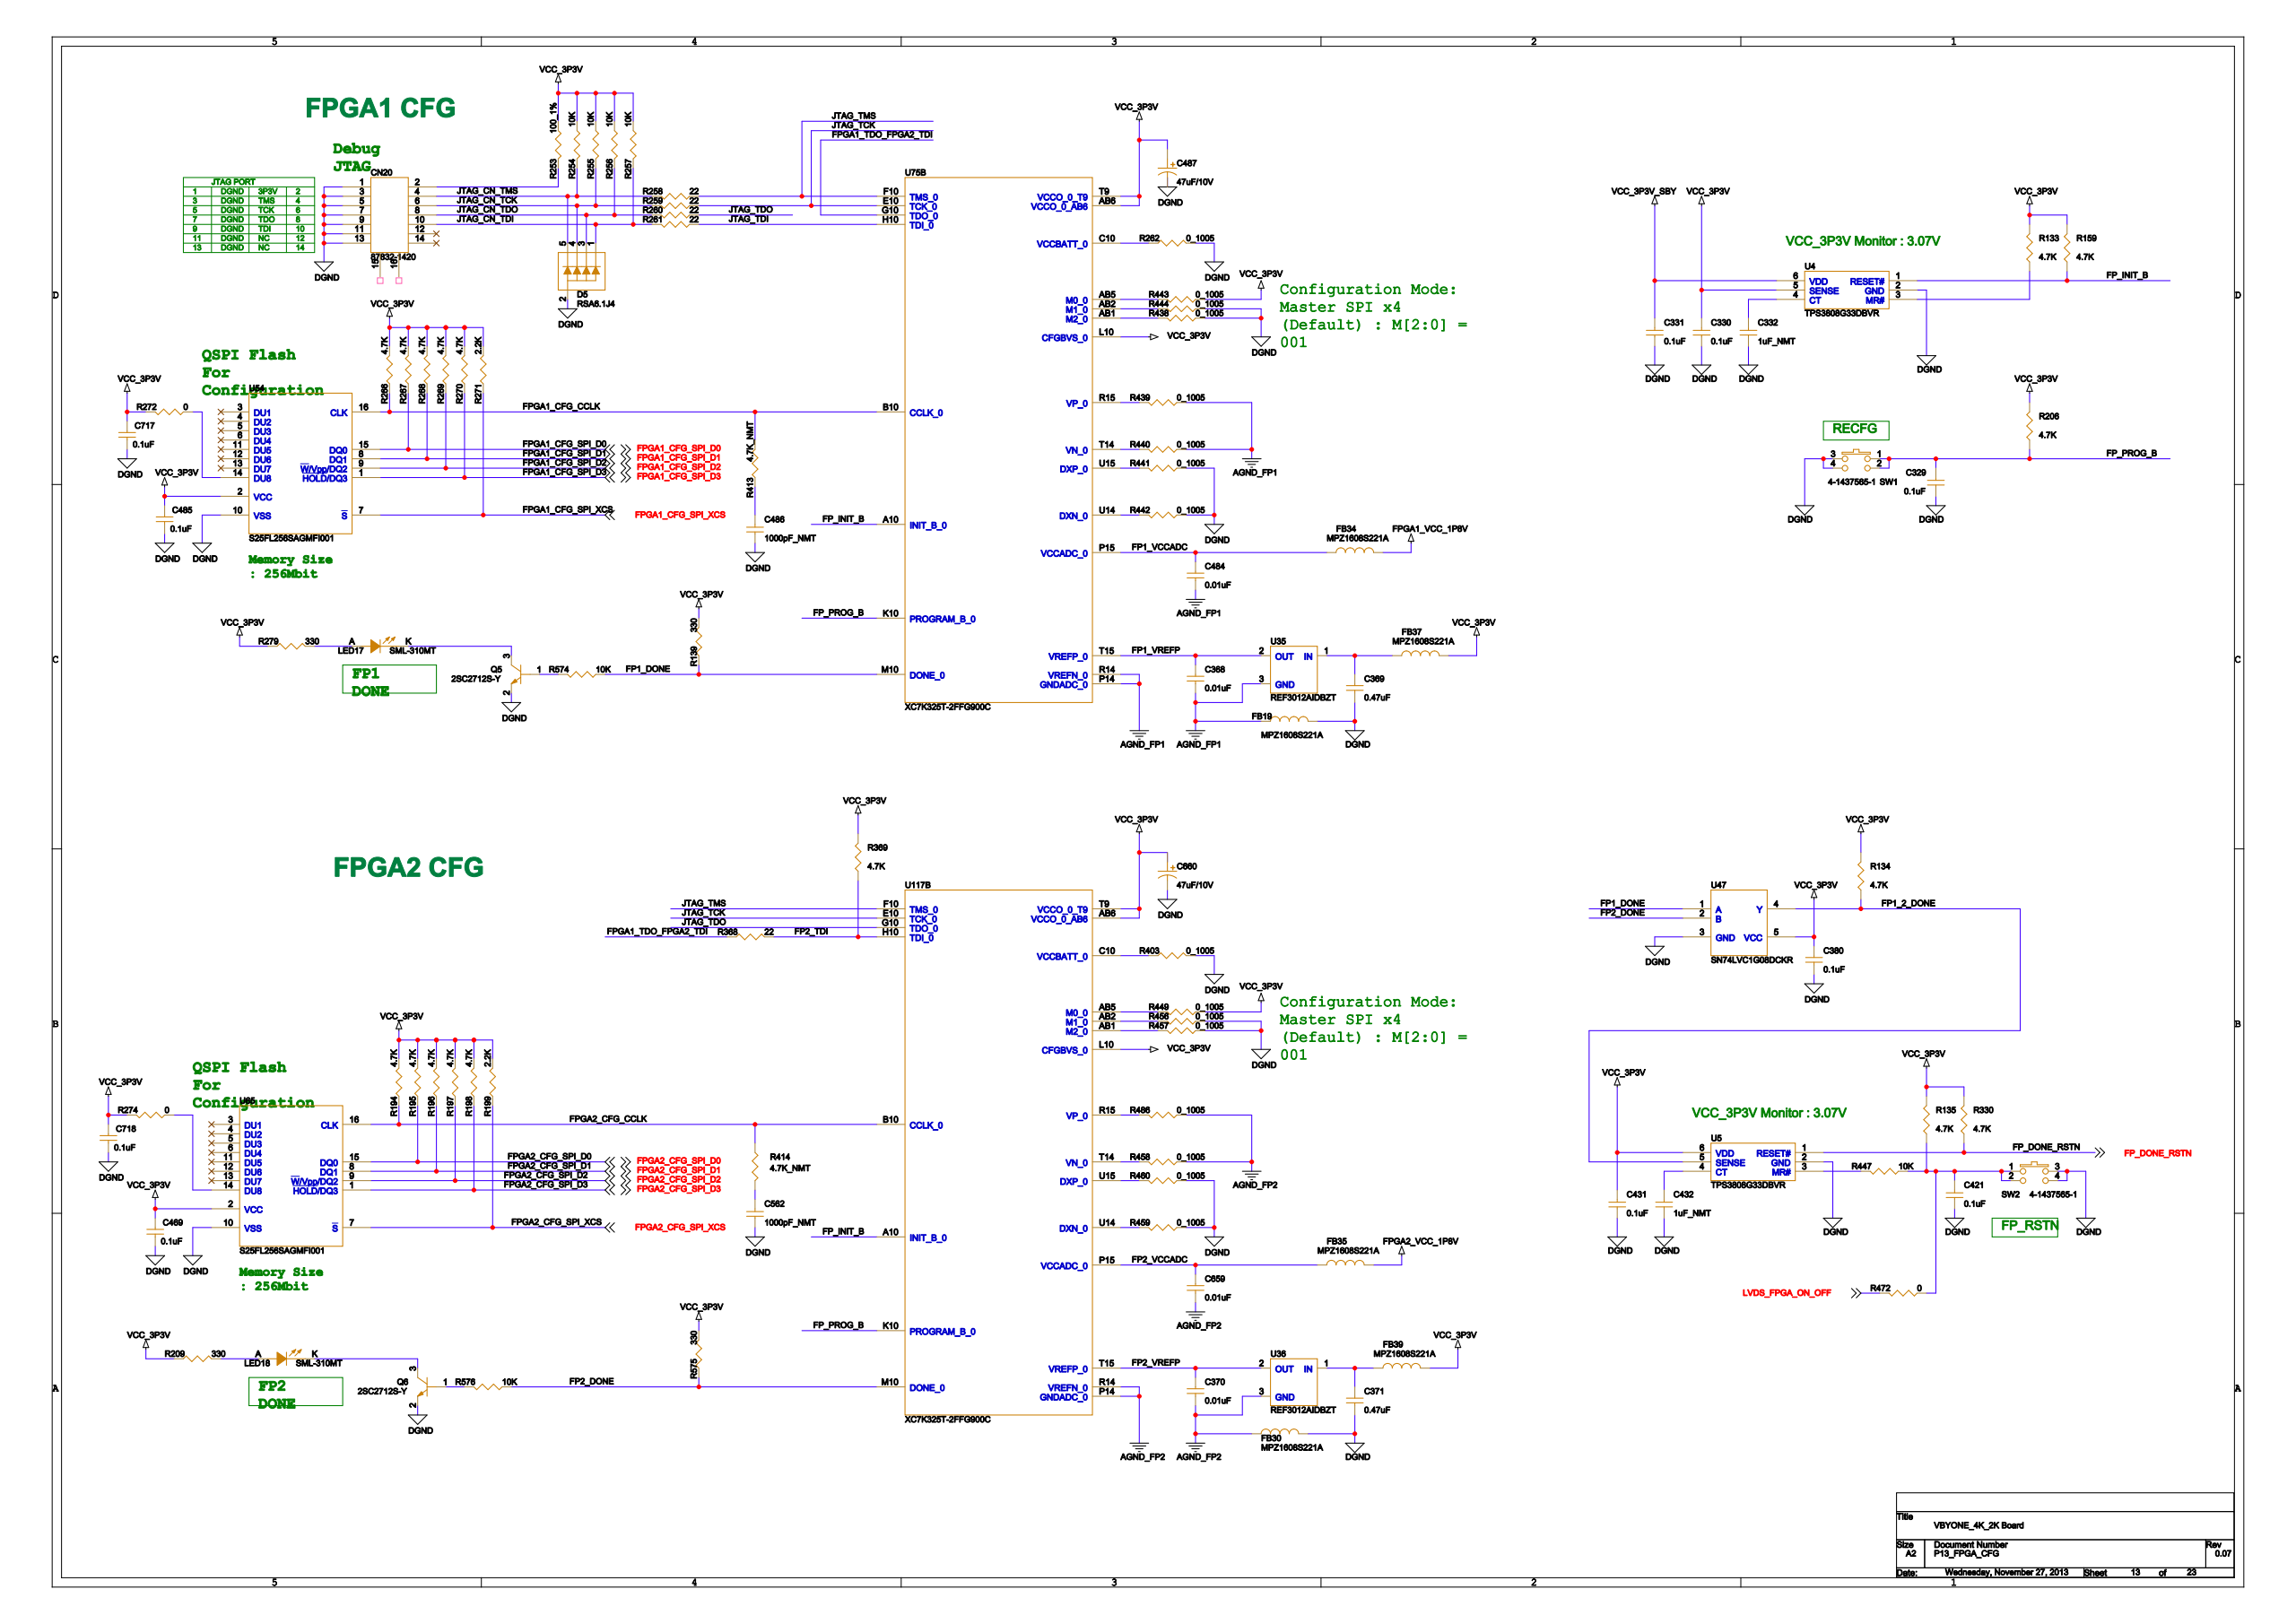Circuit board | Cadence Allegro | 1712 parts | 1495 nets | one sheet of the schematic
Parts on this sheet (reference | value | footprint):
C329 | 0.1uF | CRC1005RZAS
C330 | 0.1uF | CRC1005RZAS
C331 | 0.1uF | CRC1005RZAS
C332 | 1uF_NMT | CRC1608RZAS
C368 | 0.01uF | CRC1005RZAS
C369 | 0.47uF | CRC1608RZAS
C370 | 0.01uF | CRC1005RZAS
C371 | 0.47uF | CRC1608RZAS
C380 | 0.1uF | CRC1005RZAS
C421 | 0.1uF | CRC1005RZAS
C431 | 0.1uF | CRC1005RZAS
C432 | 1uF_NMT | CRC1608RZAS
C469 | 0.1uF | CRC1005RZAS
C484 | 0.01uF | CRC1005RZAS
C485 | 0.1uF | CRC1005RZAS
C486 | 1000pF_NMT | CRC1608RZAS
C487 | 47uF/10V | CEC3528RZAS
C562 | 1000pF_NMT | CRC1608RZAS
C659 | 0.01uF | CRC1005RZAS
C660 | 47uF/10V | CEC3528RZAS
C717 | 0.1uF | CRC1005RZAS
C718 | 0.1uF | CRC1005RZAS
CN20 | 87832-1420 | CNC014RJAS
D5 | RSA6.1J4 | DIC005RCAS
FB19 | MPZ1608S221A | LSC1608RZAS
FB30 | MPZ1608S221A | LSC1608RZAS
FB34 | MPZ1608S221A | LSC1608RZAS
FB35 | MPZ1608S221A | LSC1608RZAS
FB37 | MPZ1608S221A | LSC1608RZAS
FB39 | MPZ1608S221A | LSC1608RZAS
LED17 | SML-310MT | LEC1608RZAS
LED18 | SML-310MT | LEC1608RZAS
Q5 | 2SC2712S-Y | TRC003RZCS
Q6 | 2SC2712S-Y | TRC003RZCS
R133 | 4.7K | CRC1005RZAS
R134 | 4.7K | CRC1005RZAS
R135 | 4.7K | CRC1005RZAS
R139 | 330 | CRC1608RZAS
R159 | 4.7K | CRC1005RZAS
R194 | 4.7K | CRC1005RZAS
R195 | 4.7K | CRC1005RZAS
R196 | 4.7K | CRC1005RZAS
R197 | 4.7K | CRC1005RZAS
R198 | 4.7K | CRC1005RZAS
R199 | 2.2K | CRC1005RZAS
R206 | 4.7K | CRC1005RZAS
R209 | 330 | CRC1608RZAS
R253 | 100_1% | CRC1005RZAS
R254 | 10K | CRC1005RZAS
R255 | 10K | CRC1005RZAS
R256 | 10K | CRC1005RZAS
R257 | 10K | CRC1005RZAS
R258 | 22 | CRC1005RZAS
R259 | 22 | CRC1005RZAS
R260 | 22 | CRC1005RZAS
R261 | 22 | CRC1005RZAS
R262 | 0_1005 | CRC1005RZAS
R266 | 4.7K | CRC1005RZAS
R267 | 4.7K | CRC1005RZAS
R268 | 4.7K | CRC1005RZAS
R269 | 4.7K | CRC1005RZAS
R270 | 4.7K | CRC1005RZAS
R271 | 2.2K | CRC1005RZAS
R272 | 0 | CRC1608RZAS
R274 | 0 | CRC1608RZAS
R279 | 330 | CRC1608RZAS
R330 | 4.7K | CRC1005RZAS
R368 | 22 | CRC1005RZAS
R369 | 4.7K | CRC1005RZAS
R403 | 0_1005 | CRC1005RZAS
R413 | 4.7K_NMT | CRC1608RZAS
R414 | 4.7K_NMT | CRC1608RZAS
R438 | 0_1005 | CRC1005RZAS
R439 | 0_1005 | CRC1005RZAS
R440 | 0_1005 | CRC1005RZAS
R441 | 0_1005 | CRC1005RZAS
R442 | 0_1005 | CRC1005RZAS
R443 | 0_1005 | CRC1005RZAS
R444 | 0_1005 | CRC1005RZAS
R447 | 10K | CRC1005RZAS
R449 | 0_1005 | CRC1005RZAS
R456 | 0_1005 | CRC1005RZAS
R457 | 0_1005 | CRC1005RZAS
R458 | 0_1005 | CRC1005RZAS
R459 | 0_1005 | CRC1005RZAS
R460 | 0_1005 | CRC1005RZAS
R472 | 0 | CRC1608RZAS
R486 | 0_1005 | CRC1005RZAS
R574 | 10K | CRC1005RZAS
R575 | 330 | CRC1608RZAS
R576 | 10K | CRC1005RZAS
SW1 | 4-1437565-1 | SWC004RZBS
SW2 | 4-1437565-1 | SWC004RZBS
U4 | TPS3808G33DBVR | SOC006RZBS
U5 | TPS3808G33DBVR | SOC006RZBS
U15 | SII1161CTU | QFP100RCBS
U35 | REF3012AIDBZT | TRC003RZGS
U36 | REF3012AIDBZT | TRC003RZGS
U47 | SN74LVC1G08DCKR | SOC005REAS
U54 | S25FL256SAGMFI001 | SOC016RHAS
U65 | S25FL256SAGMFI001 | SOC016RHAS
U75 | XC7K325T-2FFG900C | BGA900RGAS
U117 | XC7K325T-2FFG900C | BGA900RGAS
Nets of these parts (net: part-pin ...):
VCC_3P3V: C330-2 C380-1 C431-2 C469-1 C485-1 C487-1 C660-1 C717-1 C718-1 FB37-2 FB39-2 R133-2 R134-2 R135-2 R139-2 R159-2 R194-1 R195-1 R196-1 R197-1 R198-1 R199-1 R206-2 R209-2 R253-2 R254-1 R255-1 R256-1 R257-1 R266-1 R267-1 R268-1 R269-1 R270-1 R271-1 R272-1 R274-1 R279-2 R330-2 R369-2 R443-1 R449-1 R575-2 U4-5 U5-6 U47-5 U54-2 U65-2 U15-2 U15-9 U75-AB6 U75-L10 U75-T9 U117-AB6 U117-L10 U117-T9
DGND: C329-1 C330-1 C331-1 C332-1 C369-2 C371-2 C380-2 C421-1 C431-1 C432-1 C469-2 C485-2 C486-1 C487-2 C562-1 C660-2 C717-2 C718-2 CN20-1 CN20-3 CN20-5 CN20-7 CN20-9 CN20-11 CN20-13 D5-2 FB19-2 FB30-2 Q5-2 Q6-2 R262-2 R403-2 R438-1 R441-1 R442-1 R444-1 R456-1 R457-1 R459-1 R460-1 SW1-3 SW1-4 SW2-3 SW2-4 U4-2 U5-2 U47-3 U54-10 U65-10 U15-5 U75-A2 U75-D5 U117-A2
VCC_3P3V_SBY: C331-2 U4-6
FPGA1_VCC_1P8V: FB34-2
FPGA2_VCC_1P8V: FB35-2
FP_PROG_B: C329-2 R206-1 SW1-1 SW1-2 U75-K10 U117-K10
N17557052: C421-2 R135-1 R447-1 R472-1 SW2-1 SW2-2
N17490659: C332-2 U4-4
N17557080: C432-2 U5-4
FP1_VREFP: C368-1 U35-2 U75-T15
AGND_FP1: C368-2 C484-2 FB19-1 R439-1 R440-1 U35-3 U75-P14 U75-R14
FP2_VREFP: C370-1 U36-2 U117-T15
AGND_FP2: C370-2 C659-2 FB30-1 R458-1 R486-1 U36-3 U117-P14 U117-R14
N18104262: C369-1 FB37-1 U35-1
N18866336: C371-1 FB39-1 U36-1
FP1_VCCADC: C484-1 FB34-1 U75-P15
FP2_VCCADC: C659-1 FB35-1 U117-P15
N18414566: C486-2 R413-2
N18867436: C562-2 R414-1
LVDS_FPGA_ON_OFF: R472-2
N17041527: CN20-2 R253-1
JTAG_CN_TMS: CN20-4 D5-5 R254-2 R258-2
JTAG_CN_TCK: CN20-6 D5-4 R255-2 R259-2
JTAG_CN_TDO: CN20-8 D5-3 R256-2 R260-2
JTAG_CN_TDI: CN20-10 D5-1 R257-2 R261-2
N17492368: LED17-A R279-1
N17492392: LED17-K Q5-3
N18869127: LED18-A R209-1
N18869143: LED18-K Q6-3
N17491683: Q5-1 R574-2
N18869112: Q6-1 R576-2
N19472699: R272-2 U54-14
N19474053: R274-2 U65-14
N18413369: R133-1 U4-3
FP1_2_DONE: R134-1 U5-5 U47-4
FP_INIT_B: R159-1 U4-1 U75-A10 U117-A10
FPGA2_CFG_CCLK: R194-2 R414-2 U65-16 U117-B10
FPGA2_CFG_SPI_D0: R195-2 U65-15
FPGA2_CFG_SPI_D1: R196-2 U65-8
FPGA2_CFG_SPI_D2: R197-2 U65-9
FPGA2_CFG_SPI_D3: R198-2 U65-1
FPGA1_CFG_CCLK: R266-2 R413-1 U54-16 U75-B10
FPGA1_CFG_SPI_D0: R267-2 U54-15
FPGA1_CFG_SPI_D1: R268-2 U54-8
FPGA1_CFG_SPI_D2: R269-2 U54-9
FPGA1_CFG_SPI_D3: R270-2 U54-1
FP_DONE_RSTN: R330-1 U5-1
FP2_TDI: R368-2 R369-1 U117-H10
N17557048: R447-2 U5-3
FP1_DONE: R139-1 R574-1 U47-1 U75-M10
FP2_DONE: R575-1 R576-1 U47-2 U117-M10
FPGA2_CFG_SPI_XCS: R199-2 U65-7
FPGA1_CFG_SPI_XCS: R271-2 U54-7
JTAG_TMS: R258-1 U75-F10 U117-F10
JTAG_TCK: R259-1 U75-E10 U117-E10
JTAG_TDO: R260-1 U117-G10
JTAG_TDI: R261-1 U75-H10
FPGA1_TDO_FPGA2_TDI: R368-1 U75-G10
N17041187: R262-1 U75-C10
N18866131: R403-1 U117-C10
N17041711: R438-2 U75-AB1
N17041997: R439-2 U75-R15
N17041298: R440-2 U75-T14
N17041825: R441-2 U75-U15
N17041816: R442-2 U75-U14
N18385016: R443-2 U75-AB5
N18385120: R444-2 U75-AB2
N18866089: R449-2 U117-AB5
N18866107: R456-2 U117-AB2
N18866222: R457-2 U117-AB1
N18866133: R458-2 U117-T14
N18866264: R459-2 U117-U14
N18866270: R460-2 U117-U15
N18866286: R486-2 U117-R15